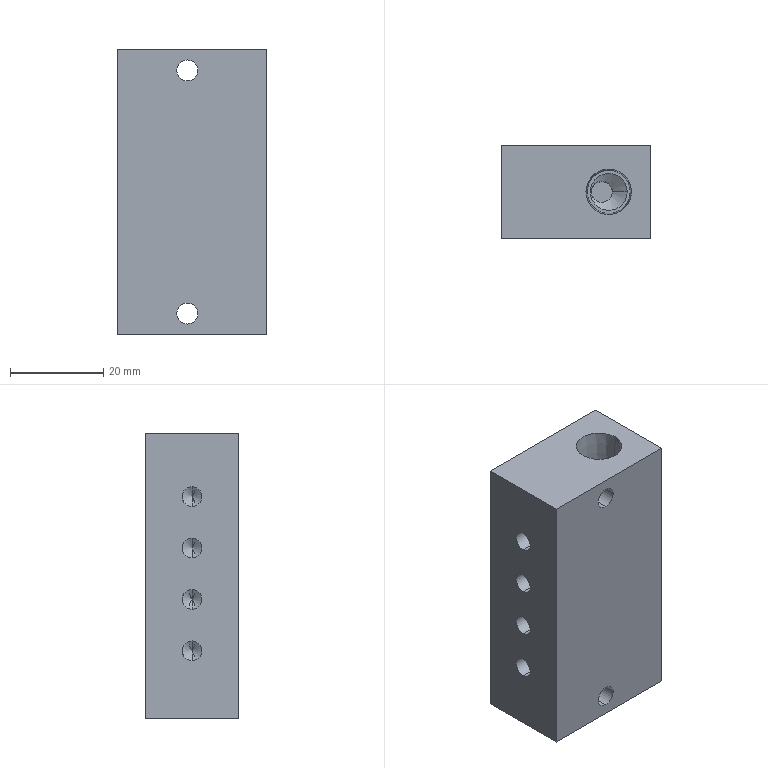Part | SolidWorks | features HoleWzd 6, ICE 5, Extrusion 1, LPattern 1, RefAxis 1, RevCut 1 | 1 solid | 116 faces | box 32 x 20 x 61 mm | volume 34864 mm3 | cylinder 64 | cone 44 | plane 8 | commonest cylinder face diameters 2 x24 1.25 x16 4.2 x16 4.5 x6 7.9 x2